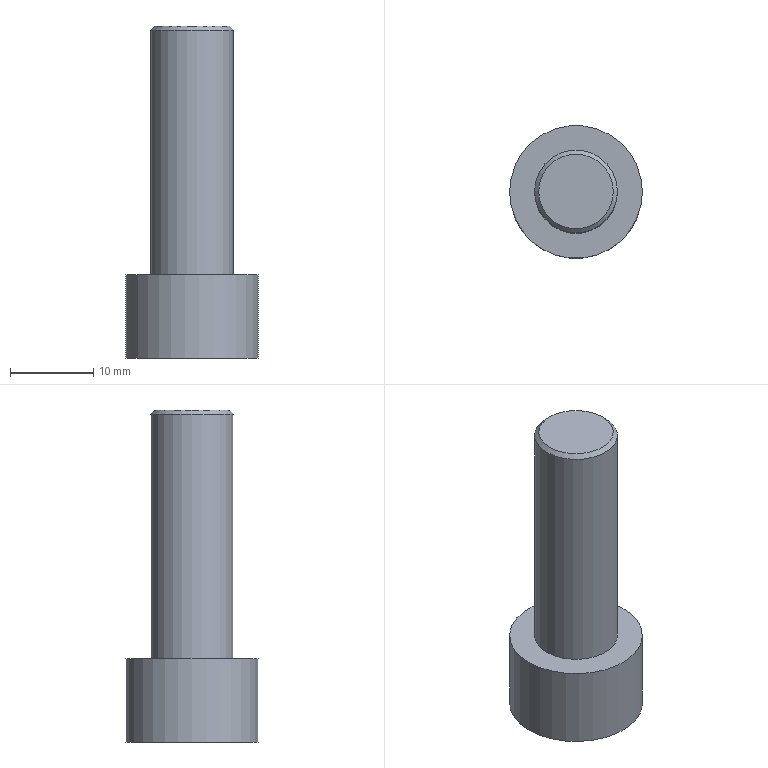Part | STEP file | PN_0057_id1198_x_t | 1 solid | 19 faces | box 16 x 16 x 40 mm | volume 4064 mm3 | plane 15 | cone 2 | cylinder 2 | commonest cylinder face diameters 10 x1 16 x1
STEP:
#1=CARTESIAN_POINT('',(233.,152.5,65.5));
#2=VERTEX_POINT('',#1);
#3=CARTESIAN_POINT('',(242.,152.5,65.5));
#4=VERTEX_POINT('',#3);
#5=CARTESIAN_POINT('',(237.5,152.5,65.5));
#6=DIRECTION('',(0.,0.,1.));
#7=DIRECTION('',(-1.,0.,0.));
#8=AXIS2_PLACEMENT_3D('',#5,#6,#7);
#9=CIRCLE('',#8,4.5);
#10=EDGE_CURVE('',#2,#4,#9,.T.);
#11=ORIENTED_EDGE('',*,*,#10,.F.);
#12=CARTESIAN_POINT('',(237.5,152.5,65.5));
#13=DIRECTION('',(0.,0.,1.));
#14=DIRECTION('',(-1.,0.,0.));
#15=AXIS2_PLACEMENT_3D('',#12,#13,#14);
#16=CIRCLE('',#15,4.5);
#17=EDGE_CURVE('',#4,#2,#16,.T.);
#18=ORIENTED_EDGE('',*,*,#17,.F.);
#19=CARTESIAN_POINT('',(242.5,152.5,65.));
#20=VERTEX_POINT('',#19);
#21=CARTESIAN_POINT('',(242.,152.5,65.5));
#22=CARTESIAN_POINT('',(242.5,152.5,65.));
#23=B_SPLINE_CURVE_WITH_KNOTS('',1,(#21,#22),.UNSPECIFIED.,.F.,.F.,(2,2),(0.,1.),.UNSPECIFIED.);
#24=EDGE_CURVE('',#4,#20,#23,.T.);
#25=ORIENTED_EDGE('',*,*,#24,.T.);
#26=CARTESIAN_POINT('',(232.5,152.5,65.));
#27=VERTEX_POINT('',#26);
#28=CARTESIAN_POINT('',(237.5,152.5,65.));
#29=DIRECTION('',(0.,0.,-1.));
#30=DIRECTION('',(-1.,0.,0.));
#31=AXIS2_PLACEMENT_3D('',#28,#29,#30);
#32=CIRCLE('',#31,5.);
#33=EDGE_CURVE('',#27,#20,#32,.T.);
#34=ORIENTED_EDGE('',*,*,#33,.F.);
#35=CARTESIAN_POINT('',(237.5,152.5,65.));
#36=DIRECTION('',(0.,0.,-1.));
#37=DIRECTION('',(-1.,0.,0.));
#38=AXIS2_PLACEMENT_3D('',#35,#36,#37);
#39=CIRCLE('',#38,5.);
#40=EDGE_CURVE('',#20,#27,#39,.T.);
#41=ORIENTED_EDGE('',*,*,#40,.F.);
#42=ORIENTED_EDGE('',*,*,#24,.F.);
#43=EDGE_LOOP('',(#11,#18,#25,#34,#41,#42));
#44=FACE_OUTER_BOUND('',#43,.T.);
#45=CARTESIAN_POINT('',(237.5,152.5,62.929));
#46=DIRECTION('',(0.,0.,-1.));
#47=DIRECTION('',(1.,0.,0.));
#48=AXIS2_PLACEMENT_3D('',#45,#46,#47);
#49=CONICAL_SURFACE('',#48,7.071,45.);
#50=ADVANCED_FACE('',(#44),#49,.T.);
#51=CARTESIAN_POINT('',(232.5,152.5,35.5));
#52=VERTEX_POINT('',#51);
#53=CARTESIAN_POINT('',(237.5,152.5,35.5));
#54=DIRECTION('',(0.,0.,1.));
#55=DIRECTION('',(-1.,0.,0.));
#56=AXIS2_PLACEMENT_3D('',#53,#54,#55);
#57=CIRCLE('',#56,5.);
#58=EDGE_CURVE('',#52,#52,#57,.T.);
#59=ORIENTED_EDGE('',*,*,#58,.T.);
#60=CARTESIAN_POINT('',(232.5,152.5,35.5));
#61=CARTESIAN_POINT('',(232.5,152.5,65.));
#62=B_SPLINE_CURVE_WITH_KNOTS('',1,(#60,#61),.UNSPECIFIED.,.F.,.F.,(2,2),(0.,1.),.UNSPECIFIED.);
#63=EDGE_CURVE('',#52,#27,#62,.T.);
#64=ORIENTED_EDGE('',*,*,#63,.T.);
#65=ORIENTED_EDGE('',*,*,#33,.T.);
#66=ORIENTED_EDGE('',*,*,#40,.T.);
#67=ORIENTED_EDGE('',*,*,#63,.F.);
#68=EDGE_LOOP('',(#59,#64,#65,#66,#67));
#69=FACE_OUTER_BOUND('',#68,.T.);
#70=CARTESIAN_POINT('',(237.5,152.5,50.5));
#71=DIRECTION('',(0.,0.,1.));
#72=DIRECTION('',(-1.,0.,0.));
#73=AXIS2_PLACEMENT_3D('',#70,#71,#72);
#74=CYLINDRICAL_SURFACE('',#73,5.);
#75=ADVANCED_FACE('',(#69),#74,.T.);
#76=ORIENTED_EDGE('',*,*,#17,.T.);
#77=ORIENTED_EDGE('',*,*,#10,.T.);
#78=EDGE_LOOP('',(#76,#77));
#79=FACE_OUTER_BOUND('',#78,.T.);
#80=CARTESIAN_POINT('',(247.85,143.147,65.5));
#81=DIRECTION('',(0.,0.,1.));
#82=DIRECTION('',(-1.,0.,0.));
#83=AXIS2_PLACEMENT_3D('',#80,#81,#82);
#84=PLANE('',#83);
#85=ADVANCED_FACE('',(#79),#84,.T.);
#86=CARTESIAN_POINT('',(237.5,147.881,30.5));
#87=VERTEX_POINT('',#86);
#88=CARTESIAN_POINT('',(233.5,150.191,30.5));
#89=VERTEX_POINT('',#88);
#90=CARTESIAN_POINT('',(237.5,147.881,30.5));
#91=DIRECTION('',(-0.866,0.5,0.));
#92=VECTOR('',#91,1.);
#93=LINE('',#90,#92);
#94=EDGE_CURVE('',#87,#89,#93,.T.);
#95=ORIENTED_EDGE('',*,*,#94,.T.);
#96=CARTESIAN_POINT('',(237.5,152.5,30.5));
#97=DIRECTION('',(0.,0.,1.));
#98=DIRECTION('',(1.,0.,0.));
#99=AXIS2_PLACEMENT_3D('',#96,#97,#98);
#100=CIRCLE('',#99,4.619);
#101=EDGE_CURVE('',#89,#87,#100,.T.);
#102=ORIENTED_EDGE('',*,*,#101,.T.);
#103=EDGE_LOOP('',(#95,#102));
#104=FACE_OUTER_BOUND('',#103,.T.);
#105=CARTESIAN_POINT('',(233.1,147.65,30.5));
#106=DIRECTION('',(0.,0.,-1.));
#107=DIRECTION('',(1.,0.,0.));
#108=AXIS2_PLACEMENT_3D('',#105,#106,#107);
#109=PLANE('',#108);
#110=ADVANCED_FACE('',(#104),#109,.F.);
#111=CARTESIAN_POINT('',(233.5,154.809,30.5));
#112=VERTEX_POINT('',#111);
#113=CARTESIAN_POINT('',(233.5,150.191,30.5));
#114=DIRECTION('',(0.,1.,0.));
#115=VECTOR('',#114,1.);
#116=LINE('',#113,#115);
#117=EDGE_CURVE('',#89,#112,#116,.T.);
#118=ORIENTED_EDGE('',*,*,#117,.T.);
#119=CARTESIAN_POINT('',(232.881,152.5,30.5));
#120=VERTEX_POINT('',#119);
#121=CARTESIAN_POINT('',(237.5,152.5,30.5));
#122=DIRECTION('',(0.,0.,1.));
#123=DIRECTION('',(1.,0.,0.));
#124=AXIS2_PLACEMENT_3D('',#121,#122,#123);
#125=CIRCLE('',#124,4.619);
#126=EDGE_CURVE('',#112,#120,#125,.T.);
#127=ORIENTED_EDGE('',*,*,#126,.T.);
#128=CARTESIAN_POINT('',(237.5,152.5,30.5));
#129=DIRECTION('',(0.,0.,1.));
#130=DIRECTION('',(1.,0.,0.));
#131=AXIS2_PLACEMENT_3D('',#128,#129,#130);
#132=CIRCLE('',#131,4.619);
#133=EDGE_CURVE('',#120,#89,#132,.T.);
#134=ORIENTED_EDGE('',*,*,#133,.T.);
#135=EDGE_LOOP('',(#118,#127,#134));
#136=FACE_OUTER_BOUND('',#135,.T.);
#137=CARTESIAN_POINT('',(232.033,149.729,30.5));
#138=DIRECTION('',(0.,0.,-1.));
#139=DIRECTION('',(1.,0.,0.));
#140=AXIS2_PLACEMENT_3D('',#137,#138,#139);
#141=PLANE('',#140);
#142=ADVANCED_FACE('',(#136),#141,.F.);
#143=CARTESIAN_POINT('',(237.5,157.119,30.5));
#144=VERTEX_POINT('',#143);
#145=CARTESIAN_POINT('',(233.5,154.809,30.5));
#146=DIRECTION('',(0.866,0.5,0.));
#147=VECTOR('',#146,1.);
#148=LINE('',#145,#147);
#149=EDGE_CURVE('',#112,#144,#148,.T.);
#150=ORIENTED_EDGE('',*,*,#149,.T.);
#151=CARTESIAN_POINT('',(237.5,152.5,30.5));
#152=DIRECTION('',(0.,0.,1.));
#153=DIRECTION('',(1.,0.,0.));
#154=AXIS2_PLACEMENT_3D('',#151,#152,#153);
#155=CIRCLE('',#154,4.619);
#156=EDGE_CURVE('',#144,#112,#155,.T.);
#157=ORIENTED_EDGE('',*,*,#156,.T.);
#158=EDGE_LOOP('',(#150,#157));
#159=FACE_OUTER_BOUND('',#158,.T.);
#160=CARTESIAN_POINT('',(233.1,154.578,30.5));
#161=DIRECTION('',(0.,0.,-1.));
#162=DIRECTION('',(1.,0.,0.));
#163=AXIS2_PLACEMENT_3D('',#160,#161,#162);
#164=PLANE('',#163);
#165=ADVANCED_FACE('',(#159),#164,.F.);
#166=CARTESIAN_POINT('',(241.5,154.809,30.5));
#167=VERTEX_POINT('',#166);
#168=CARTESIAN_POINT('',(237.5,157.119,30.5));
#169=DIRECTION('',(0.866,-0.5,0.));
#170=VECTOR('',#169,1.);
#171=LINE('',#168,#170);
#172=EDGE_CURVE('',#144,#167,#171,.T.);
#173=ORIENTED_EDGE('',*,*,#172,.T.);
#174=CARTESIAN_POINT('',(237.5,152.5,30.5));
#175=DIRECTION('',(0.,0.,1.));
#176=DIRECTION('',(1.,0.,0.));
#177=AXIS2_PLACEMENT_3D('',#174,#175,#176);
#178=CIRCLE('',#177,4.619);
#179=EDGE_CURVE('',#167,#144,#178,.T.);
#180=ORIENTED_EDGE('',*,*,#179,.T.);
#181=EDGE_LOOP('',(#173,#180));
#182=FACE_OUTER_BOUND('',#181,.T.);
#183=CARTESIAN_POINT('',(237.1,154.578,30.5));
#184=DIRECTION('',(0.,0.,-1.));
#185=DIRECTION('',(1.,0.,0.));
#186=AXIS2_PLACEMENT_3D('',#183,#184,#185);
#187=PLANE('',#186);
#188=ADVANCED_FACE('',(#182),#187,.F.);
#189=CARTESIAN_POINT('',(241.5,150.191,30.5));
#190=VERTEX_POINT('',#189);
#191=CARTESIAN_POINT('',(241.5,154.809,30.5));
#192=DIRECTION('',(0.,-1.,0.));
#193=VECTOR('',#192,1.);
#194=LINE('',#191,#193);
#195=EDGE_CURVE('',#167,#190,#194,.T.);
#196=ORIENTED_EDGE('',*,*,#195,.T.);
#197=CARTESIAN_POINT('',(237.5,152.5,30.5));
#198=DIRECTION('',(0.,0.,1.));
#199=DIRECTION('',(0.866,-0.5,0.));
#200=AXIS2_PLACEMENT_3D('',#197,#198,#199);
#201=CIRCLE('',#200,4.619);
#202=EDGE_CURVE('',#190,#167,#201,.T.);
#203=ORIENTED_EDGE('',*,*,#202,.T.);
#204=EDGE_LOOP('',(#196,#203));
#205=FACE_OUTER_BOUND('',#204,.T.);
#206=CARTESIAN_POINT('',(241.367,149.729,30.5));
#207=DIRECTION('',(0.,0.,-1.));
#208=DIRECTION('',(1.,0.,0.));
#209=AXIS2_PLACEMENT_3D('',#206,#207,#208);
#210=PLANE('',#209);
#211=ADVANCED_FACE('',(#205),#210,.F.);
#212=CARTESIAN_POINT('',(241.5,150.191,30.5));
#213=DIRECTION('',(-0.866,-0.5,0.));
#214=VECTOR('',#213,1.);
#215=LINE('',#212,#214);
#216=EDGE_CURVE('',#190,#87,#215,.T.);
#217=ORIENTED_EDGE('',*,*,#216,.T.);
#218=CARTESIAN_POINT('',(237.5,152.5,30.5));
#219=DIRECTION('',(0.,0.,1.));
#220=DIRECTION('',(1.,0.,0.));
#221=AXIS2_PLACEMENT_3D('',#218,#219,#220);
#222=CIRCLE('',#221,4.619);
#223=EDGE_CURVE('',#87,#190,#222,.T.);
#224=ORIENTED_EDGE('',*,*,#223,.T.);
#225=EDGE_LOOP('',(#217,#224));
#226=FACE_OUTER_BOUND('',#225,.T.);
#227=CARTESIAN_POINT('',(237.1,147.65,30.5));
#228=DIRECTION('',(0.,0.,-1.));
#229=DIRECTION('',(1.,0.,0.));
#230=AXIS2_PLACEMENT_3D('',#227,#228,#229);
#231=PLANE('',#230);
#232=ADVANCED_FACE('',(#226),#231,.F.);
#233=ORIENTED_EDGE('',*,*,#126,.F.);
#234=ORIENTED_EDGE('',*,*,#156,.F.);
#235=ORIENTED_EDGE('',*,*,#179,.F.);
#236=ORIENTED_EDGE('',*,*,#202,.F.);
#237=ORIENTED_EDGE('',*,*,#223,.F.);
#238=ORIENTED_EDGE('',*,*,#101,.F.);
#239=ORIENTED_EDGE('',*,*,#133,.F.);
#240=CARTESIAN_POINT('',(237.5,152.5,31.5));
#241=VERTEX_POINT('',#240);
#242=CARTESIAN_POINT('',(237.5,152.5,31.5));
#243=CARTESIAN_POINT('',(232.881,152.5,30.5));
#244=B_SPLINE_CURVE_WITH_KNOTS('',1,(#242,#243),.UNSPECIFIED.,.F.,.F.,(2,2),(0.,1.),.UNSPECIFIED.);
#245=EDGE_CURVE('',#241,#120,#244,.T.);
#246=ORIENTED_EDGE('',*,*,#245,.F.);
#247=ORIENTED_EDGE('',*,*,#245,.T.);
#248=EDGE_LOOP('',(#233,#234,#235,#236,#237,#238,#239,#246,#247));
#249=FACE_OUTER_BOUND('',#248,.T.);
#250=CARTESIAN_POINT('',(237.5,152.5,30.086));
#251=DIRECTION('',(0.,0.,-1.));
#252=DIRECTION('',(-1.,0.,0.));
#253=AXIS2_PLACEMENT_3D('',#250,#251,#252);
#254=CONICAL_SURFACE('',#253,6.532,77.784);
#255=ADVANCED_FACE('',(#249),#254,.F.);
#256=CARTESIAN_POINT('',(237.5,147.881,25.5));
#257=VERTEX_POINT('',#256);
#258=CARTESIAN_POINT('',(237.5,147.881,30.5));
#259=DIRECTION('',(0.,0.,-1.));
#260=VECTOR('',#259,1.);
#261=LINE('',#258,#260);
#262=EDGE_CURVE('',#87,#257,#261,.T.);
#263=ORIENTED_EDGE('',*,*,#262,.T.);
#264=CARTESIAN_POINT('',(233.5,150.191,25.5));
#265=VERTEX_POINT('',#264);
#266=CARTESIAN_POINT('',(237.5,147.881,25.5));
#267=DIRECTION('',(-0.866,0.5,0.));
#268=VECTOR('',#267,1.);
#269=LINE('',#266,#268);
#270=EDGE_CURVE('',#257,#265,#269,.T.);
#271=ORIENTED_EDGE('',*,*,#270,.T.);
#272=CARTESIAN_POINT('',(233.5,150.191,30.5));
#273=DIRECTION('',(0.,0.,-1.));
#274=VECTOR('',#273,1.);
#275=LINE('',#272,#274);
#276=EDGE_CURVE('',#89,#265,#275,.T.);
#277=ORIENTED_EDGE('',*,*,#276,.F.);
#278=ORIENTED_EDGE('',*,*,#94,.F.);
#279=EDGE_LOOP('',(#263,#271,#277,#278));
#280=FACE_OUTER_BOUND('',#279,.T.);
#281=CARTESIAN_POINT('',(237.9,147.65,25.));
#282=DIRECTION('',(0.5,0.866,0.));
#283=DIRECTION('',(0.,0.,1.));
#284=AXIS2_PLACEMENT_3D('',#281,#282,#283);
#285=PLANE('',#284);
#286=ADVANCED_FACE('',(#280),#285,.T.);
#287=CARTESIAN_POINT('',(241.5,150.191,25.5));
#288=VERTEX_POINT('',#287);
#289=CARTESIAN_POINT('',(241.5,150.191,30.5));
#290=DIRECTION('',(0.,0.,-1.));
#291=VECTOR('',#290,1.);
#292=LINE('',#289,#291);
#293=EDGE_CURVE('',#190,#288,#292,.T.);
#294=ORIENTED_EDGE('',*,*,#293,.T.);
#295=CARTESIAN_POINT('',(241.5,150.191,25.5));
#296=DIRECTION('',(-0.866,-0.5,0.));
#297=VECTOR('',#296,1.);
#298=LINE('',#295,#297);
#299=EDGE_CURVE('',#288,#257,#298,.T.);
#300=ORIENTED_EDGE('',*,*,#299,.T.);
#301=ORIENTED_EDGE('',*,*,#262,.F.);
#302=ORIENTED_EDGE('',*,*,#216,.F.);
#303=EDGE_LOOP('',(#294,#300,#301,#302));
#304=FACE_OUTER_BOUND('',#303,.T.);
#305=CARTESIAN_POINT('',(237.1,147.65,31.));
#306=DIRECTION('',(-0.5,0.866,0.));
#307=DIRECTION('',(0.,0.,-1.));
#308=AXIS2_PLACEMENT_3D('',#305,#306,#307);
#309=PLANE('',#308);
#310=ADVANCED_FACE('',(#304),#309,.T.);
#311=CARTESIAN_POINT('',(241.5,154.809,25.5));
#312=VERTEX_POINT('',#311);
#313=CARTESIAN_POINT('',(241.5,154.809,30.5));
#314=DIRECTION('',(0.,0.,-1.));
#315=VECTOR('',#314,1.);
#316=LINE('',#313,#315);
#317=EDGE_CURVE('',#167,#312,#316,.T.);
#318=ORIENTED_EDGE('',*,*,#317,.T.);
#319=CARTESIAN_POINT('',(241.5,154.809,25.5));
#320=DIRECTION('',(0.,-1.,0.));
#321=VECTOR('',#320,1.);
#322=LINE('',#319,#321);
#323=EDGE_CURVE('',#312,#288,#322,.T.);
#324=ORIENTED_EDGE('',*,*,#323,.T.);
#325=ORIENTED_EDGE('',*,*,#293,.F.);
#326=ORIENTED_EDGE('',*,*,#195,.F.);
#327=EDGE_LOOP('',(#318,#324,#325,#326));
#328=FACE_OUTER_BOUND('',#327,.T.);
#329=CARTESIAN_POINT('',(241.5,149.729,31.));
#330=DIRECTION('',(-1.,0.,0.));
#331=DIRECTION('',(0.,0.,-1.));
#332=AXIS2_PLACEMENT_3D('',#329,#330,#331);
#333=PLANE('',#332);
#334=ADVANCED_FACE('',(#328),#333,.T.);
#335=CARTESIAN_POINT('',(237.5,157.119,25.5));
#336=VERTEX_POINT('',#335);
#337=CARTESIAN_POINT('',(237.5,157.119,30.5));
#338=DIRECTION('',(0.,0.,-1.));
#339=VECTOR('',#338,1.);
#340=LINE('',#337,#339);
#341=EDGE_CURVE('',#144,#336,#340,.T.);
#342=ORIENTED_EDGE('',*,*,#341,.T.);
#343=CARTESIAN_POINT('',(237.5,157.119,25.5));
#344=DIRECTION('',(0.866,-0.5,0.));
#345=VECTOR('',#344,1.);
#346=LINE('',#343,#345);
#347=EDGE_CURVE('',#336,#312,#346,.T.);
#348=ORIENTED_EDGE('',*,*,#347,.T.);
#349=ORIENTED_EDGE('',*,*,#317,.F.);
#350=ORIENTED_EDGE('',*,*,#172,.F.);
#351=EDGE_LOOP('',(#342,#348,#349,#350));
#352=FACE_OUTER_BOUND('',#351,.T.);
#353=CARTESIAN_POINT('',(241.9,154.578,31.));
#354=DIRECTION('',(-0.5,-0.866,0.));
#355=DIRECTION('',(0.,0.,-1.));
#356=AXIS2_PLACEMENT_3D('',#353,#354,#355);
#357=PLANE('',#356);
#358=ADVANCED_FACE('',(#352),#357,.T.);
#359=CARTESIAN_POINT('',(233.5,154.809,25.5));
#360=VERTEX_POINT('',#359);
#361=CARTESIAN_POINT('',(233.5,154.809,30.5));
#362=DIRECTION('',(0.,0.,-1.));
#363=VECTOR('',#362,1.);
#364=LINE('',#361,#363);
#365=EDGE_CURVE('',#112,#360,#364,.T.);
#366=ORIENTED_EDGE('',*,*,#365,.T.);
#367=CARTESIAN_POINT('',(233.5,154.809,25.5));
#368=DIRECTION('',(0.866,0.5,0.));
#369=VECTOR('',#368,1.);
#370=LINE('',#367,#369);
#371=EDGE_CURVE('',#360,#336,#370,.T.);
#372=ORIENTED_EDGE('',*,*,#371,.T.);
#373=ORIENTED_EDGE('',*,*,#341,.F.);
#374=ORIENTED_EDGE('',*,*,#149,.F.);
#375=EDGE_LOOP('',(#366,#372,#373,#374));
#376=FACE_OUTER_BOUND('',#375,.T.);
#377=CARTESIAN_POINT('',(233.1,154.578,25.));
#378=DIRECTION('',(0.5,-0.866,0.));
#379=DIRECTION('',(0.,0.,1.));
#380=AXIS2_PLACEMENT_3D('',#377,#378,#379);
#381=PLANE('',#380);
#382=ADVANCED_FACE('',(#376),#381,.T.);
#383=ORIENTED_EDGE('',*,*,#276,.T.);
#384=CARTESIAN_POINT('',(233.5,150.191,25.5));
#385=DIRECTION('',(0.,1.,0.));
#386=VECTOR('',#385,1.);
#387=LINE('',#384,#386);
#388=EDGE_CURVE('',#265,#360,#387,.T.);
#389=ORIENTED_EDGE('',*,*,#388,.T.);
#390=ORIENTED_EDGE('',*,*,#365,.F.);
#391=ORIENTED_EDGE('',*,*,#117,.F.);
#392=EDGE_LOOP('',(#383,#389,#390,#391));
#393=FACE_OUTER_BOUND('',#392,.T.);
#394=CARTESIAN_POINT('',(233.5,149.729,25.));
#395=DIRECTION('',(1.,0.,0.));
#396=DIRECTION('',(0.,0.,1.));
#397=AXIS2_PLACEMENT_3D('',#394,#395,#396);
#398=PLANE('',#397);
#399=ADVANCED_FACE('',(#393),#398,.T.);
#400=CARTESIAN_POINT('',(229.5,152.5,25.5));
#401=VERTEX_POINT('',#400);
#402=CARTESIAN_POINT('',(237.5,152.5,25.5));
#403=DIRECTION('',(0.,0.,1.));
#404=DIRECTION('',(-1.,0.,0.));
#405=AXIS2_PLACEMENT_3D('',#402,#403,#404);
#406=CIRCLE('',#405,8.);
#407=EDGE_CURVE('',#401,#401,#406,.T.);
#408=ORIENTED_EDGE('',*,*,#407,.T.);
#409=CARTESIAN_POINT('',(229.5,152.5,35.5));
#410=VERTEX_POINT('',#409);
#411=CARTESIAN_POINT('',(229.5,152.5,25.5));
#412=CARTESIAN_POINT('',(229.5,152.5,35.5));
#413=B_SPLINE_CURVE_WITH_KNOTS('',1,(#411,#412),.UNSPECIFIED.,.F.,.F.,(2,2),(0.,1.),.UNSPECIFIED.);
#414=EDGE_CURVE('',#401,#410,#413,.T.);
#415=ORIENTED_EDGE('',*,*,#414,.T.);
#416=CARTESIAN_POINT('',(237.5,152.5,35.5));
#417=DIRECTION('',(0.,0.,-1.));
#418=DIRECTION('',(-1.,0.,0.));
#419=AXIS2_PLACEMENT_3D('',#416,#417,#418);
#420=CIRCLE('',#419,8.);
#421=EDGE_CURVE('',#410,#410,#420,.T.);
#422=ORIENTED_EDGE('',*,*,#421,.T.);
#423=ORIENTED_EDGE('',*,*,#414,.F.);
#424=EDGE_LOOP('',(#408,#415,#422,#423));
#425=FACE_OUTER_BOUND('',#424,.T.);
#426=CARTESIAN_POINT('',(237.5,152.5,30.5));
#427=DIRECTION('',(0.,0.,1.));
#428=DIRECTION('',(-1.,0.,0.));
#429=AXIS2_PLACEMENT_3D('',#426,#427,#428);
#430=CYLINDRICAL_SURFACE('',#429,8.);
#431=ADVANCED_FACE('',(#425),#430,.T.);
#432=ORIENTED_EDGE('',*,*,#407,.F.);
#433=EDGE_LOOP('',(#432));
#434=FACE_BOUND('',#433,.T.);
#435=ORIENTED_EDGE('',*,*,#270,.F.);
#436=ORIENTED_EDGE('',*,*,#299,.F.);
#437=ORIENTED_EDGE('',*,*,#323,.F.);
#438=ORIENTED_EDGE('',*,*,#347,.F.);
#439=ORIENTED_EDGE('',*,*,#371,.F.);
#440=ORIENTED_EDGE('',*,*,#388,.F.);
#441=EDGE_LOOP('',(#435,#436,#437,#438,#439,#440));
#442=FACE_BOUND('',#441,.T.);
#443=CARTESIAN_POINT('',(227.1,135.872,25.5));
#444=DIRECTION('',(0.,0.,-1.));
#445=DIRECTION('',(1.,0.,0.));
#446=AXIS2_PLACEMENT_3D('',#443,#444,#445);
#447=PLANE('',#446);
#448=ADVANCED_FACE('',(#434,#442),#447,.T.);
#449=ORIENTED_EDGE('',*,*,#421,.F.);
#450=EDGE_LOOP('',(#449));
#451=FACE_BOUND('',#450,.T.);
#452=ORIENTED_EDGE('',*,*,#58,.F.);
#453=EDGE_LOOP('',(#452));
#454=FACE_BOUND('',#453,.T.);
#455=CARTESIAN_POINT('',(255.9,135.872,35.5));
#456=DIRECTION('',(0.,0.,1.));
#457=DIRECTION('',(-1.,0.,0.));
#458=AXIS2_PLACEMENT_3D('',#455,#456,#457);
#459=PLANE('',#458);
#460=ADVANCED_FACE('',(#451,#454),#459,.T.);
#461=CLOSED_SHELL('',(#50,#75,#85,#110,#142,#165,#188,#211,#232,#255,#286,#310,#334,#358,#382,#399,#431,#448,#460));
#462=MANIFOLD_SOLID_BREP('',#461);
#463=(LENGTH_UNIT()NAMED_UNIT(*)SI_UNIT(.MILLI.,.METRE.));
#464=UNCERTAINTY_MEASURE_WITH_UNIT(LENGTH_MEASURE(0.00002),#463,'','');
#465=(NAMED_UNIT(*)PLANE_ANGLE_UNIT()SI_UNIT($,.RADIAN.));
#466=PLANE_ANGLE_MEASURE_WITH_UNIT(PLANE_ANGLE_MEASURE(0.01745),#465);
#467=DIMENSIONAL_EXPONENTS(0.,0.,0.,0.,0.,0.,0.);
#468=(CONVERSION_BASED_UNIT('DEGREE',#466)NAMED_UNIT(#467)PLANE_ANGLE_UNIT());
#469=(NAMED_UNIT(*)SI_UNIT($,.STERADIAN.)SOLID_ANGLE_UNIT());
#470=(GEOMETRIC_REPRESENTATION_CONTEXT(3)GLOBAL_UNCERTAINTY_ASSIGNED_CONTEXT((#464))GLOBAL_UNIT_ASSIGNED_CONTEXT((#463,#468,#469))REPRESENTATION_CONTEXT('',''));
#471=ADVANCED_BREP_SHAPE_REPRESENTATION('',(#462),#470);